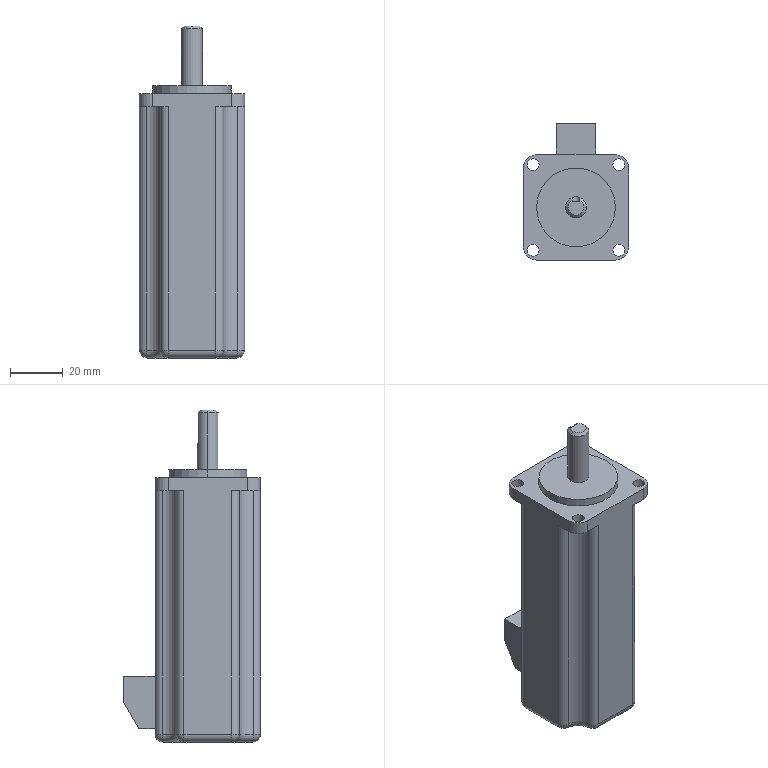Part | SolidWorks | features ICE 5, Fillet 4, Chamfer 2, Extrusion 1, HoleWzd 1 | 1 solid | 69 faces | box 40 x 52 x 126.15 mm | volume 143595 mm3 | cylinder 33 | plane 21 | sphere 8 | torus 4 | cone 3 | commonest cylinder face diameters 6 x12 4.5 x8 10 x4 12 x4 8 x2 30 x2